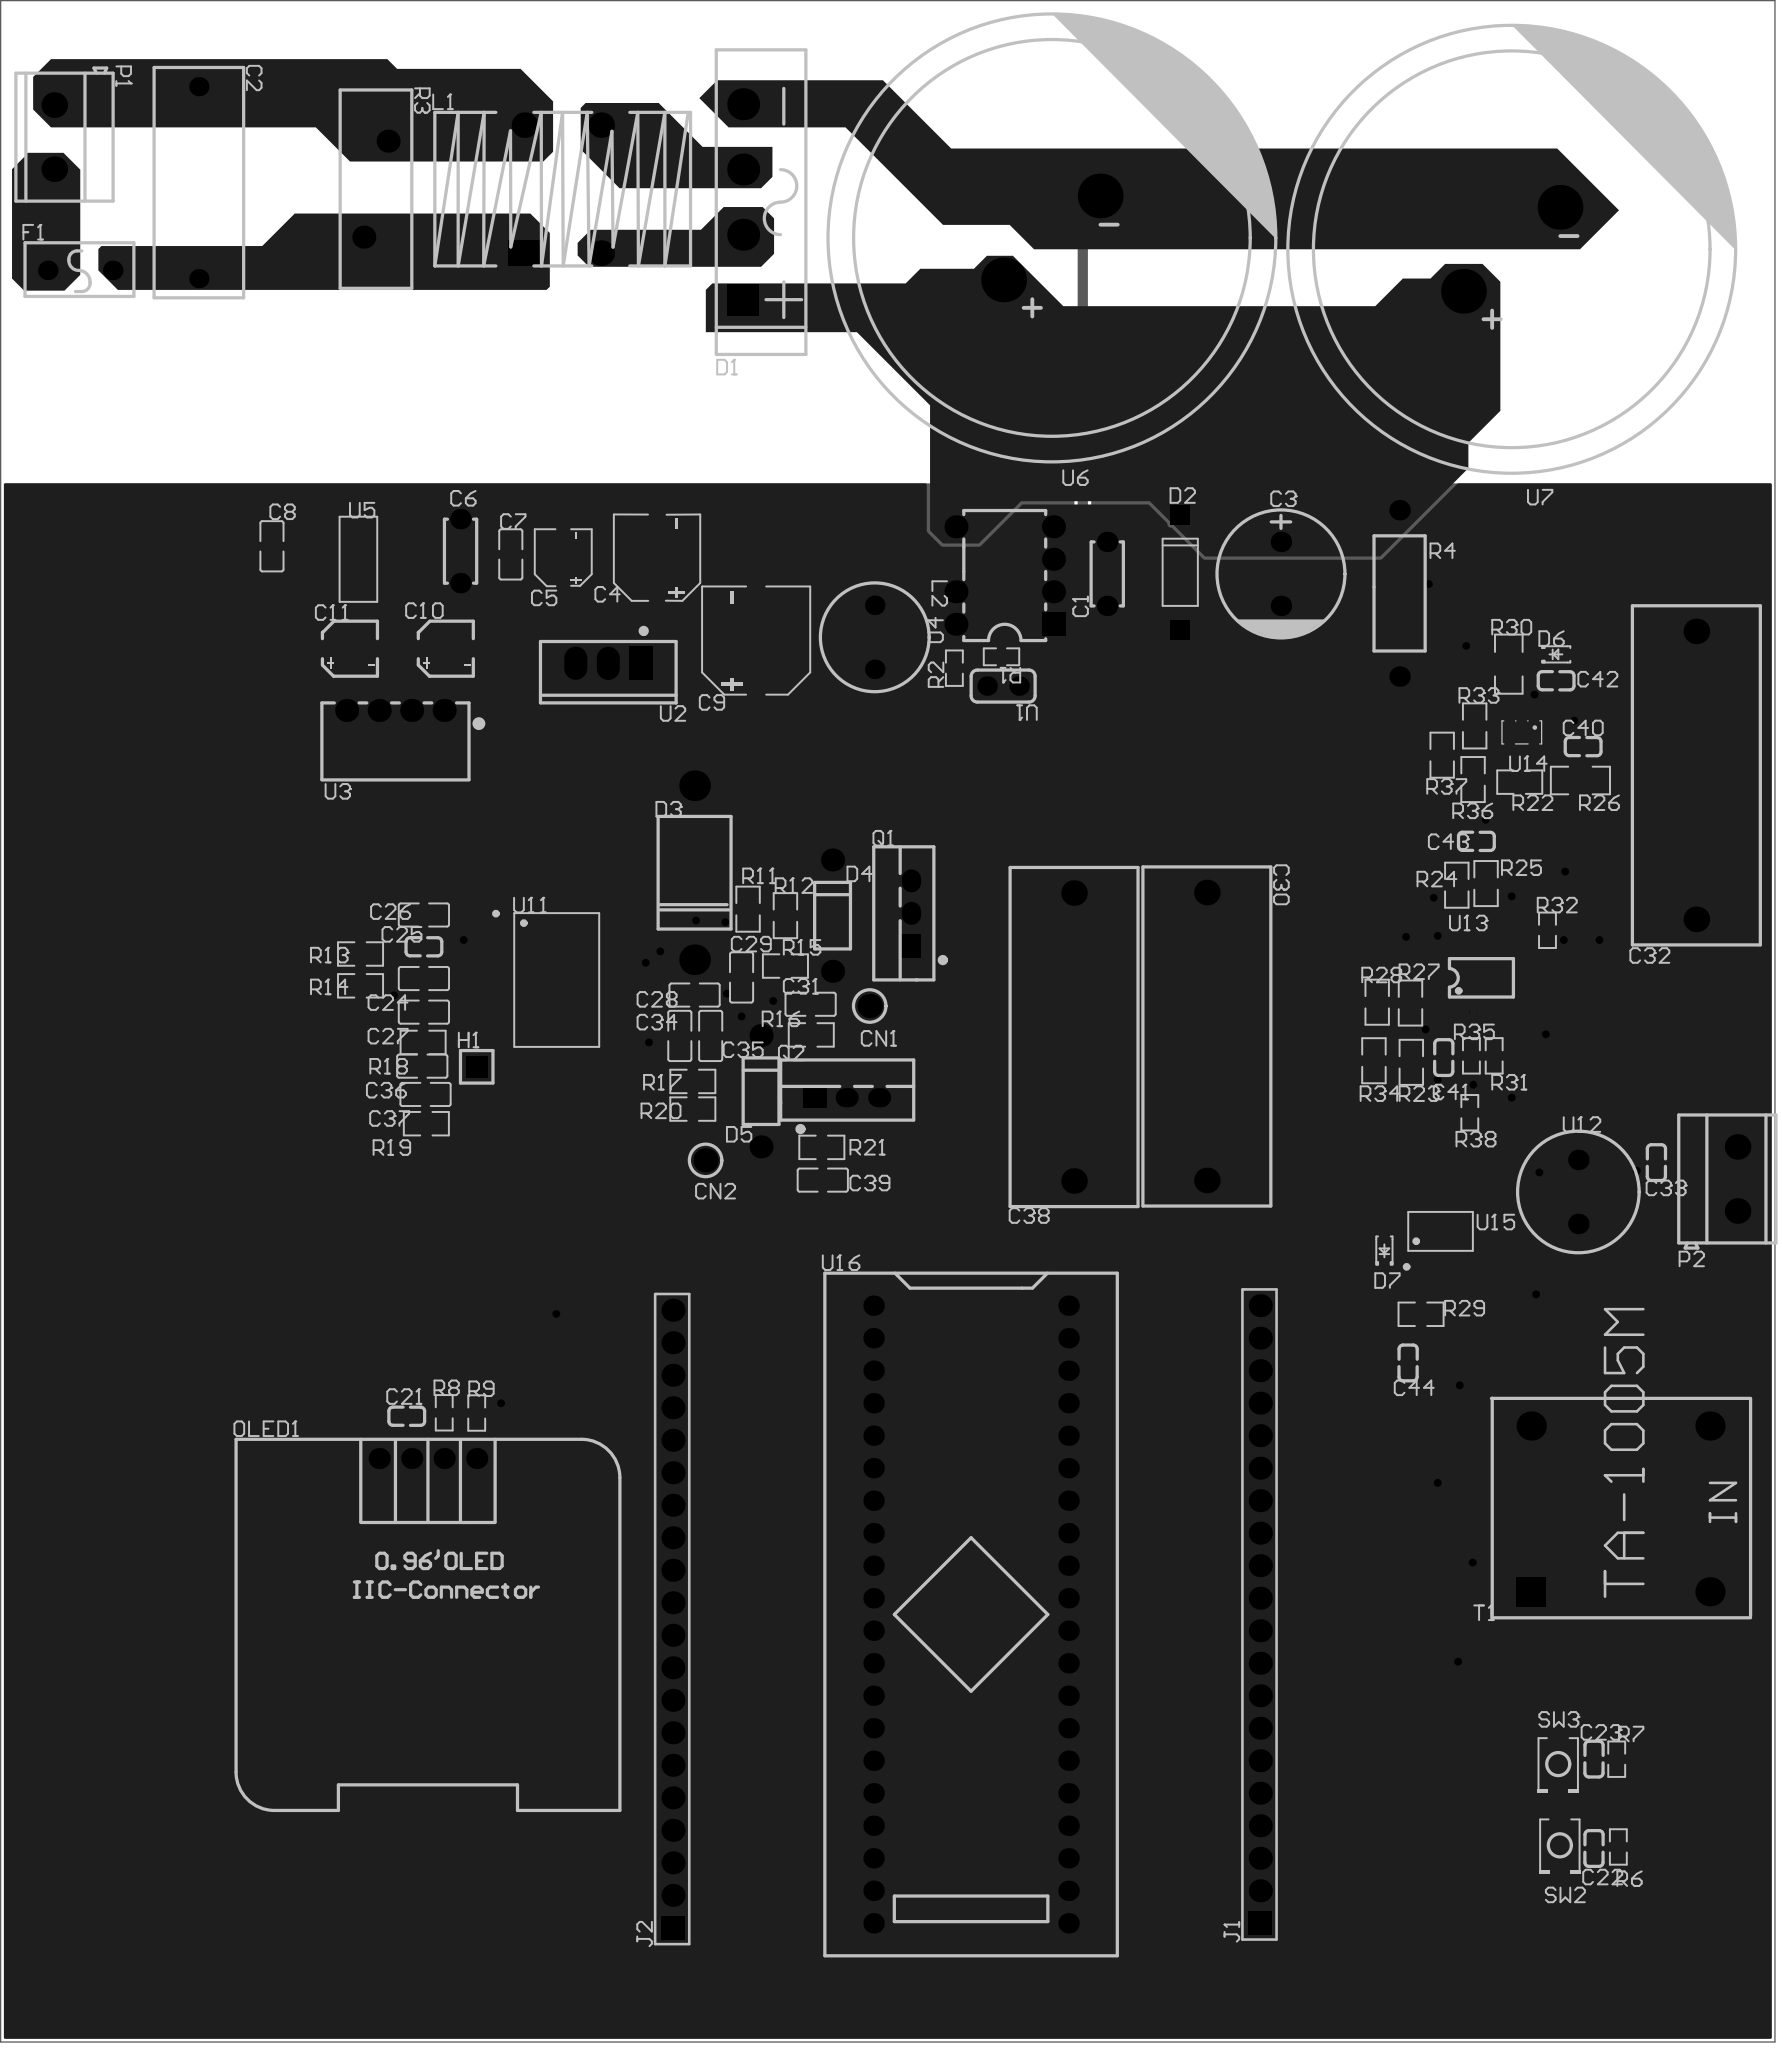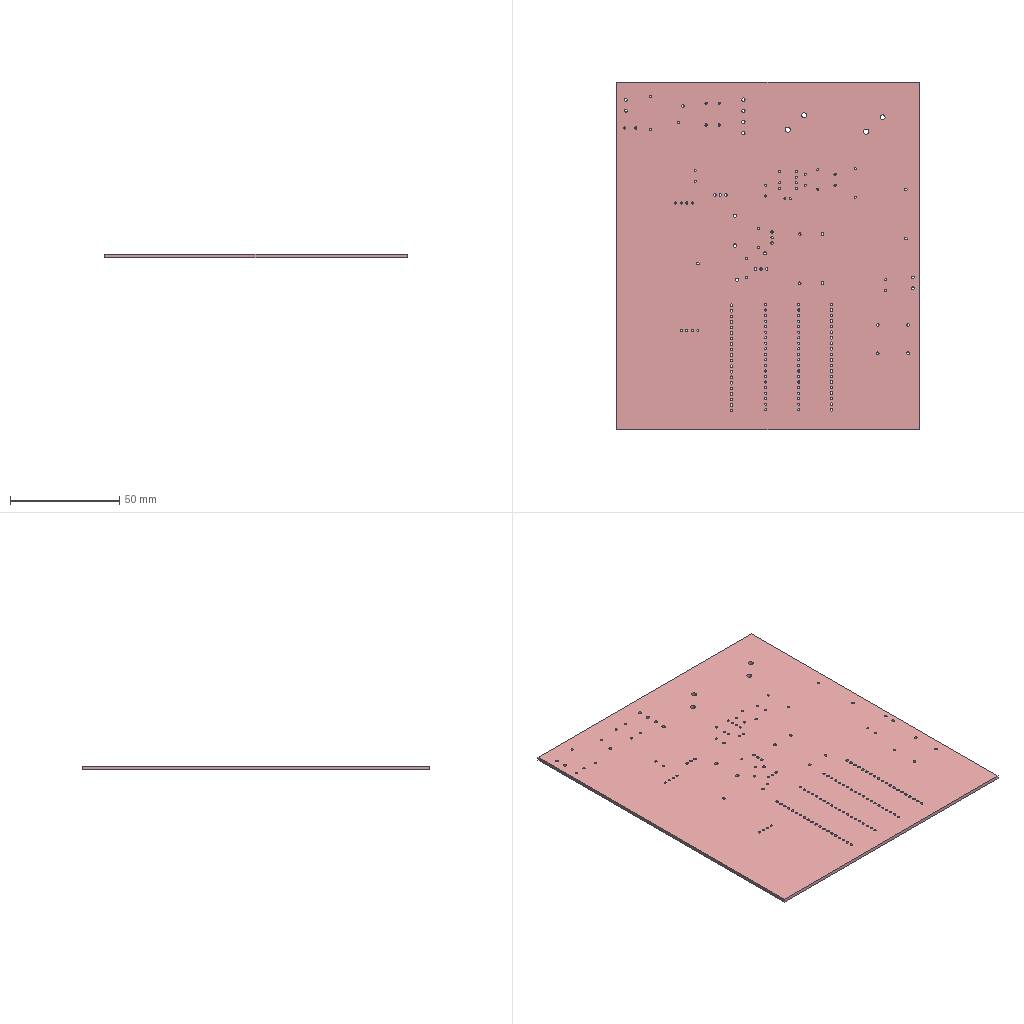Circuit board layout | Altium Designer | box 138.7 x 159.5 x 1.6 mm
Layer stack:
# Altium Designer layer stack of  (unit mm; dielectric type: 0 none, 1 core, 2 prepreg, 3 surface material)
index,name,kind,layer,copper_thickness_mm,dielectric_type,dielectric_thickness_mm,dielectric_material,dielectric_constant
0,Top Paste Mask Layer,other,,,,,,
1,Top Silkscreen Layer,other,,,,,,
2,Top Solder Mask Layer,dielectric,,,3,0.01,,3.3
3,Top Layer,copper,Top Layer,0.035,,,,
4,Dielectric1,dielectric,,,3,1.51,FR4,4.5
5,Bottom Layer,copper,Bottom Layer,0.035,,,,
6,Bottom Solder Mask Layer,dielectric,,,3,0.01,,3.3
7,Bottom Silkscreen Layer,other,,,,,,
8,Bottom Paste Mask Layer,other,,,,,,
# drill layer pairs: low layer,high layer
drill_pair,Top Layer,Bottom Layer
Part placement:
Designator,Comment,Layer,Footprint,Center-X(mm),Center-Y(mm),Rotation
C1,100nF,TopLayer,CAP-TH_L5.0-W2.5-P5.00-D1.0,183.639,198.789,90
C2,330nF,TopLayer,CAP-TH_L18.0-W7.0-P15.00-D0.7,112.649,229.362,270
C3,10uF,TopLayer,CAP-TH_BD10.0-P5.00-D0.6-FD_1,197.228,198.789,270
C4,100uF,TopLayer,CAP-SMD_BD6.3-L6.6-W6.6-FD,148.46,200.059,90
C5,10uF,TopLayer,CAP-SMD_BD4.0-L4.3-W4.3-FD,141.13,200.044,90
C6,100nF,TopLayer,CAP-TH_L5.0-W2.5-P5.00-D1.0,133.093,200.567,90
C7,10uF,TopLayer,C0805,137.03,200.313,270
C8,10uF,TopLayer,C0805,118.361,200.948,270
C9,470uF,TopLayer,CAP-SMD_BD8.0-L8.3-W8.3-LS9.2-FD-H10.5,156.207,193.582,90
C10,10uF,TopLayer,CAP-SMD_BD4.0-L4.3-W4.3-FD_1,131.95,192.947,0
C11,10uF,TopLayer,CAP-SMD_BD4.0-L4.3-W4.3-FD_1,124.457,192.947,0
C21,100nF,TopLayer,C0603,128.905,132.969,0
C22,100nF,TopLayer,C0603,221.692,99.187,270
C23,100nF,TopLayer,C0603,221.692,106.172,270
C24,10uF,TopLayer,C0805,130.238,167.171,0
C25,100nF,TopLayer,C0603,130.245,169.652,0
C26,22PF,TopLayer,C0805,130.238,172.137,180
C27,22PF,TopLayer,C0805,130.238,164.548,0
C28,100nf,TopLayer,C0805,151.395,165.883,0
C29,2.2uf,TopLayer,C0805,155.067,167.259,270
C30,10uF/630V CBB,TopLayer,1uf/630V_CBB,191.436,162.645,270
C31,1nf,TopLayer,C0805,160.463,165.162,0
C32,10uF/630V CBB,TopLayer,1uf/630V_CBB,229.696,183.049,90
C33,100nF,TopLayer,C0603,226.568,152.781,270
C34,100nF,TopLayer,C0805,150.241,162.687,270
C35,2.2uf,TopLayer,C0805,152.654,162.687,270
C36,22pf,TopLayer,C0805,130.111,160.327,0
C37,100nF,TopLayer,C0805,130.365,158.115,0
C38,10uF/630V CBB,TopLayer,1uf/630V_CBB,181.055,162.602,90
C39,1nf,TopLayer,C0805,161.415,151.421,180
C40,100nF,TopLayer,C0603,220.853,185.293,0
C41,100nF,TopLayer,C0603,209.955,161.004,90
C42,100nF,TopLayer,C0603,218.726,190.442,180
C43,100nF,TopLayer,C0603,212.495,177.895,180
C44,100nF,TopLayer,C0603,207.161,137.128,270
CN1,RH-5001,TopLayer,TEST-TH_BD2.54-P1.4_BLACK,165.083,165.025,0
CN2,RH-5001,TopLayer,TEST-TH_BD2.54-P1.4_BLACK,152.256,152.96,0
D1,KBU810,TopLayer,DIO-BG-TH_L23.2-W6.8-P5.10_KBU,155.194,227.838,270
D2,BYV26C,TopLayer,DO-41_BD2.6-L5.1-P9.00-D0.8-RD,189.354,198.916,270
D3,SR5100,TopLayer,DO-201AD_BD5.3-L8.4-P12.50-D1.4-RD,151.395,175.44,90
D4,1N5819,TopLayer,DO-41_BD2.4-L4.7-P8.70-D0.9-FD,162.179,172.085,90
D5,1N5819,TopLayer,DO-41_BD2.4-L4.7-P8.70-D0.9-FD,156.591,158.369,90
D6,BZT52C3V3S,TopLayer,SOD-323_L1.7-W1.3-LS2.6-RD,218.718,192.5,0
D7,BZT52C3V3S,TopLayer,SOD-323_L1.7-W1.3-LS2.6-RD,205.312,145.894,90
F1,MTS1315A,TopLayer,FUSE-TH_L8.4-W4.0-P5.08-D0.6,103.378,222.504,0
H1,PZ254V-11-01P,TopLayer,HDR-TH_1P-P2.54-V-M,134.366,160.274,0
J1,2.54-1*20P直针,TopLayer,HDR-TH_20P-P2.54-V-M-1,195.612,117.48,90
J2,2.54-1*20P直针,TopLayer,HDR-TH_20P-P2.54-V-M-1,149.708,117.122,90
L1,PDMCAT16128-103ML,TopLayer,IND-TH_4P-L20.0-W12.0-P6.00-LS10.0-BL,141.097,228.854,0
L2,1mH,TopLayer,IND-TH_BD8.5-P5.00-D0.6,165.478,193.836,270
OLED1,,TopLayer,0.96OLED_4P,130.556,129.667,0
P1,CONN-TH_2P-P5.00,TopLayer,CONN-TH_2P-P5.00,101.346,232.918,270
P2,CONN-TH_2P-P5.00,TopLayer,CONN-TH_2P-P5.00,232.918,151.511,90
Q1,IRF840,TopLayer,TO-220-3_L10.2-W4.5-P2.54-L-1,168.348,172.264,90
Q2,IRF840,TopLayer,TO-220-3_L10.2-W4.5-P2.54-L-1,163.322,157.861,0
R1,6.2kΩ,TopLayer,R0603,175.384,192.312,180
R2,20kΩ,TopLayer,R0603,171.701,191.423,90
R3,420pF@1kHz,TopLayer,RES-TH_L15.5-W5.6-P7.50-D0.8-S1.90,126.492,228.854,270
R4,220kΩ,TopLayer,RES-TH_BD3.9-L9.0-P13.00-D0.8,206.499,197.265,90
R6,10kΩ,TopLayer,R0603_1,223.597,99.314,90
R7,10kΩ,TopLayer,R0603_1,223.47,106.172,90
R8,4.7kΩ,TopLayer,R0603,131.826,133.24,90
R9,4.7kΩ,TopLayer,R0603,134.366,133.223,90
R11,4.7R,TopLayer,R0805,155.575,172.593,90
R12,4.7R,TopLayer,R0805,158.496,172.085,90
R13,47R,TopLayer,R0805,125.285,169.089,0
R14,47R,TopLayer,R0805,125.285,166.603,0
R15,10r,TopLayer,R0805,158.496,168.148,180
R16,10K,TopLayer,R0805,160.515,162.766,0
R17,4.7R,TopLayer,R0805,151.257,159.131,0
R18,10K,TopLayer,R0805,130.175,162.179,0
R19,4.7k,TopLayer,R0805,130.429,155.829,0
R20,10r,TopLayer,R0805,151.257,156.972,180
R21,10K,TopLayer,R0805,161.341,153.978,180
R22,10kΩ,TopLayer,R0805,215.89,182.518,180
R23,10kΩ,TopLayer,R0805,207.415,160.623,90
R24,10kΩ,TopLayer,R0805,210.971,174.466,270
R25,10kΩ,TopLayer,R0805,213.257,174.593,270
R26,1MΩ,TopLayer,R1206,220.634,182.645,180
R27,100Ω,TopLayer,R0805,207.352,165.259,270
R28,10kΩ,TopLayer,R0805,204.748,165.322,90
R29,820Ω,TopLayer,R0805,208.177,140.938,0
R30,1MΩ,TopLayer,R1206,215.035,191.738,270
R31,1kΩ,TopLayer,R0603,213.892,161.131,90
R32,1kΩ,TopLayer,R0603,218.059,170.942,270
R33,10kΩ,TopLayer,R0805,212.368,186.912,90
R34,100Ω,TopLayer,R0805,204.494,160.75,90
R35,100kΩ,TopLayer,R0603,212.114,161.131,270
R36,10kΩ,TopLayer,R0805,212.241,182.721,270
R37,10kΩ,TopLayer,R0805,209.828,184.626,90
R38,3.3kΩ,TopLayer,R0603_NEW,211.987,156.686,90
SW2,TS-1088-AR02016,TopLayer,SW-SMD_L3.9-W3.0-P4.45,219.025,99.441,270
SW3,TS-1088-AR02016,TopLayer,SW-SMD_L3.9-W3.0-P4.45,218.898,105.791,270
T1,TA-1005M,TopLayer,TA-1005M,223.774,125.73,90
U1,10nF,TopLayer,CAP-TH_L5.0-W2.5-P2.50-D0.5,175.511,190.026,180
U2,LM7805,TopLayer,TO-220-3_L10.0-W4.5-P2.54-L,144.65,191.804,180
U3,260kHz,TopLayer,PWRM-TH_4P-L11.5-W6.0-P2.54_B1503S,128.013,188.121,180
U4,LNK304PN,TopLayer,DIP-8_7P-L9.7-W6.4-P2.54-LS7.6-BL-PE6,175.638,198.662,90
U5,AMS1117-3.3,TopLayer,SOT-223-3_L6.5-W3.4-P2.30-LS7.0-BR,125.219,199.932,0
U6,470uF,TopLayer,CAP-TH_BD35.0-P10.00-D1.5-FD,179.324,225.044,0
U7,470uF,TopLayer,CAP-TH_BD35.0-P10.00-D1.5-FD,215.265,224.155,0
U11,UCC21520ADWR,TopLayer,SOIC-16_L10.3-W7.5-P1.27-LS10.3-BL,140.618,167.058,270
U12,2.5mH,TopLayer,IND-TH_BD9.5-P5.00-D0.7,220.472,150.495,270
U13,LM393DR,TopLayer,SOIC-8_L5.0-W4.0-P1.27-LS6.0-BL,212.896,167.227,0
U14,AD8605ARTZ-REEL7,TopLayer,SOT-23-5_L3.0-W1.7-P0.95-LS2.8-BR,216.051,186.404,90
U15,LM358DT,TopLayer,SOIC-8_L4.9-W3.9-P1.27-LS6.0-BL,209.701,147.415,0
U16,STM32F103C8T6-Card,TopLayer,CONN-TH_L53.3-W22.9_STM32F103C8T6-CARD,173.006,117.48,270
Pad and via stacks:
# Altium Designer via and pad stacks of  (unit mm). Each distinct definition once, with the count of objects using it.
# via: kind,start_layer,end_layer,hole_mm,diameter_mm,mode(0 simple;1 top-mid-bottom;2 full stack),diameter_per_layer,count,example_net
# pad: kind,layer,hole_mm,hole_type(0 round;1 square;2 slot),plating,top_size,top_shape(1 round;2 rect;3 octagon;9 rounded rect),mid_size,bottom_size,mode,footprint,size_per_layer,count,example
pad,Multi-Layer,1,0,plated,1.6x1.6,1,1.6x1.6,1.6x1.6,0,CAP-TH_L5.0-W2.5-P5.00-D1.0,,4,C1.1
pad,Multi-Layer,1,0,plated,1.5x1.5,1,1.5x1.5,1.5x1.5,0,CAP-TH_L18.0-W7.0-P15.00-D0.7,,2,C2.1
pad,Multi-Layer,1,0,plated,1.6x1.6,1,1.6x1.6,1.6x1.6,0,CAP-TH_BD10.0-P5.00-D0.6-FD_1,,2,C3.2
pad,Multi-Layer,1.2,0,plated,2x2,1,2x2,2x2,0,1uf/630V CBB,,6,C30.1
pad,Multi-Layer,1.39,0,plated,1.9x1.9,1,1.9x1.9,1.9x1.9,0,TEST-TH_BD2.54-P1.4_BLACK,,2,CN1.1
pad,Multi-Layer,1.6,0,plated,2.5x2.5,2,2.5x2.5,2.5x2.5,0,DIO-BG-TH_L23.2-W6.8-P5.10_KBU,,1,D1.1
pad,Multi-Layer,1.6,0,plated,2.5x2.5,1,2.5x2.5,2.5x2.5,0,DIO-BG-TH_L23.2-W6.8-P5.10_KBU,,3,D1.2
pad,Multi-Layer,1,0,plated,1.5x1.5,2,1.5x1.5,1.5x1.5,0,DO-41_BD2.6-L5.1-P9.00-D0.8-RD,,2,D2.1
pad,Multi-Layer,1.6,0,plated,2.4x2.4,1,2.4x2.4,2.4x2.4,0,DO-201AD_BD5.3-L8.4-P12.50-D1.4-RD,,2,D3.2
pad,Multi-Layer,1,0,plated,1.8x1.8,1,1.8x1.8,1.8x1.8,0,DO-41_BD2.4-L4.7-P8.70-D0.9-FD,,4,D4.1
pad,Multi-Layer,1,0,plated,1.524x1.524,1,1.524x1.524,1.524x1.524,0,FUSE-TH_L8.4-W4.0-P5.08-D0.6,,2,F1.1
pad,Multi-Layer,1.1,0,plated,1.7x1.7,2,1.7x1.7,1.7x1.7,0,HDR-TH_1P-P2.54-V-M,,1,H1.1
pad,Multi-Layer,1.2,0,plated,1.8x1.8,1,1.8x1.8,1.8x1.8,0,HDR-TH_20P-P2.54-V-M-1,,38,J1.20
pad,Multi-Layer,1.2,0,plated,1.8x1.8,2,1.8x1.8,1.8x1.8,0,HDR-TH_20P-P2.54-V-M-1,,2,J1.1
pad,Multi-Layer,1,0,plated,2x2,1,2x2,2x2,0,IND-TH_4P-L20.0-W12.0-P6.00-LS10.0-BL,,3,L1.4
pad,Multi-Layer,1,0,plated,2.5x2,2,2.5x2,2.5x2,0,IND-TH_4P-L20.0-W12.0-P6.00-LS10.0-BL,,1,L1.1
pad,Multi-Layer,1,0,plated,1.524x1.524,1,1.524x1.524,1.524x1.524,0,IND-TH_BD8.5-P5.00-D0.6,,2,L2.1
pad,Multi-Layer,1,0,plated,1.65x1.65,1,1.65x1.65,1.65x1.65,0,0.96OLED_4P,,4,OLED1.4
pad,Multi-Layer,1.3,0,plated,2x2,1,2x2,2x2,0,CONN-TH_2P-P5.00,,4,P1.1
pad,Multi-Layer,1,2,plated,1.8x1.5,2,1.8x1.5,1.8x1.5,0,TO-220-3_L10.2-W4.5-P2.54-L-1,,2,Q1.1
pad,Multi-Layer,1,2,plated,1.8x1.5,1,1.8x1.5,1.8x1.5,0,TO-220-3_L10.2-W4.5-P2.54-L-1,,4,Q1.3
pad,Multi-Layer,1.2,0,plated,1.8x1.8,1,1.8x1.8,1.8x1.8,0,RES-TH_L15.5-W5.6-P7.50-D0.8-S1.90,,2,R3.1
pad,Multi-Layer,1,0,plated,1.6x1.6,1,1.6x1.6,1.6x1.6,0,RES-TH_BD3.9-L9.0-P13.00-D0.8,,2,R4.2
pad,Multi-Layer,1.226,0,plated,2.286x2.286,2,2.286x2.286,2.286x2.286,0,TA-1005M,,1,T1.4
pad,Multi-Layer,1.2,0,plated,2.286x2.286,1,2.286x2.286,2.286x2.286,0,TA-1005M,,3,T1.1
pad,Multi-Layer,0.9144,0,plated,1.524x1.524,1,1.524x1.524,1.524x1.524,0,CAP-TH_L5.0-W2.5-P2.50-D0.5,,2,U1.1
pad,Multi-Layer,1.2,0,plated,1.8x2.6,1,1.8x2.6,1.8x2.6,0,TO-220-3_L10.0-W4.5-P2.54-L,,2,U2.2
pad,Multi-Layer,1.2,0,plated,1.8x2.6,2,1.8x2.6,1.8x2.6,0,TO-220-3_L10.0-W4.5-P2.54-L,,1,U2.1
pad,Multi-Layer,1,0,plated,1.8x1.8,1,1.8x1.8,1.8x1.8,0,PWRM-TH_4P-L11.5-W6.0-P2.54_B1503S,,4,U3.4
pad,Multi-Layer,1,0,plated,1.8x1.8,1,1.8x1.8,1.8x1.8,0,DIP-8_7P-L9.7-W6.4-P2.54-LS7.6-BL-PE6,,6,U4.8
pad,Multi-Layer,1,0,plated,1.8x1.8,2,1.8x1.8,1.8x1.8,0,DIP-8_7P-L9.7-W6.4-P2.54-LS7.6-BL-PE6,,1,U4.1
pad,Multi-Layer,2.3,0,plated,3.5x3.5,1,3.5x3.5,3.5x3.5,0,CAP-TH_BD35.0-P10.00-D1.5-FD,,4,U6.2
pad,Multi-Layer,0.9,0,plated,1.6x1.6,1,1.6x1.6,1.6x1.6,0,IND-TH_BD9.5-P5.00-D0.7,,2,U12.1
pad,Multi-Layer,1,0,plated,1.6x1.6,1,1.6x1.6,1.6x1.6,0,CONN-TH_L53.3-W22.9_STM32F103C8T6-CARD,,40,U16.1
pad,Top Layer,0,0,plated,3.5x1.2,2,3.5x1.2,3.5x1.2,0,CAP-SMD_BD6.3-L6.6-W6.6-FD,,2,C4.1
pad,Top Layer,0,0,plated,2.8x1.1,2,2.8x1.1,2.8x1.1,0,CAP-SMD_BD4.0-L4.3-W4.3-FD,,2,C5.1
pad,Top Layer,0,0,plated,1.41x1.35,2,1.41x1.35,1.41x1.35,0,C0805,,26,C7.2
pad,Top Layer,0,0,plated,3.61x1.26,2,3.61x1.26,3.61x1.26,0,CAP-SMD_BD8.0-L8.3-W8.3-LS9.2-FD-H10.5,,2,C9.1
pad,Top Layer,0,0,plated,2.6x1.1,2,2.6x1.1,2.6x1.1,0,CAP-SMD_BD4.0-L4.3-W4.3-FD_1,,4,C10.2
pad,Top Layer,0,0,plated,0.8x0.9,2,0.8x0.9,0.8x0.9,0,C0603,,20,C21.2
pad,Top Layer,0,0,plated,0.63x0.83,2,0.63x0.83,0.63x0.83,0,SOD-323_L1.7-W1.3-LS2.6-RD,,4,D6.2
pad,Top Layer,0,0,plated,0.8065x0.864,2,0.8065x0.864,0.8065x0.864,0,R0603,,14,R1.2
pad,Top Layer,0,0,plated,0.8065x0.864,2,0.8065x0.864,0.8065x0.864,0,R0603_1,,4,R6.2
pad,Top Layer,0,0,plated,1.133x1.377,2,1.133x1.377,1.133x1.377,0,R0805,,44,R11.2
pad,Top Layer,0,0,plated,1.208x1.701,2,1.208x1.701,1.208x1.701,0,R1206,,4,R26.2
pad,Top Layer,0,0,plated,0.8065x0.864,2,0.8065x0.864,0.8065x0.864,0,R0603_NEW,,2,R38.2
pad,Top Layer,0,0,plated,1.23x1.36,2,1.23x1.36,1.23x1.36,0,SW-SMD_L3.9-W3.0-P4.45,,4,SW2.1
pad,Top Layer,0,0,plated,2.5x1.1,2,2.5x1.1,2.5x1.1,0,SOT-223-3_L6.5-W3.4-P2.30-LS7.0-BR,,3,U5.1
pad,Top Layer,0,0,plated,2.34x3.6,2,2.34x3.6,2.34x3.6,0,SOT-223-3_L6.5-W3.4-P2.30-LS7.0-BR,,1,U5.4
pad,Top Layer,0,0,plated,0.574x2.401,1,0.574x2.401,0.574x2.401,0,SOIC-16_L10.3-W7.5-P1.27-LS10.3-BL,,16,U11.1
pad,Top Layer,0,0,plated,0.5684x1.95,1,0.5684x1.95,0.5684x1.95,0,SOIC-8_L5.0-W4.0-P1.27-LS6.0-BL,,8,U13.1
pad,Top Layer,0,0,plated,1.1x0.6,2,1.1x0.6,1.1x0.6,0,SOT-23-5_L3.0-W1.7-P0.95-LS2.8-BR,,5,U14.5
pad,Top Layer,0,0,plated,0.588x2.045,1,0.588x2.045,0.588x2.045,0,SOIC-8_L4.9-W3.9-P1.27-LS6.0-BL,,8,U15.1
via,Top Layer,Bottom Layer,0.3048,0.61,0,,37,3V3
Copper pours:
name,layer,net,type(0 solid;1 hatched;2 none)
Bottom Layer-GND,Bottom Layer,GND,0
Top Layer-GND,Top Layer,GND,0